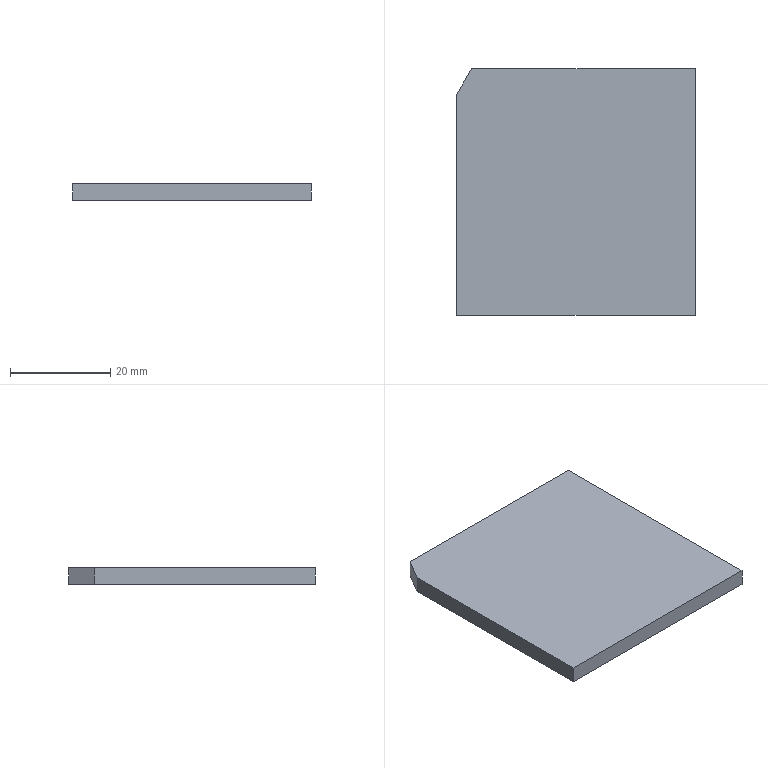Part | SolidWorks | features BaseBody 1 | 1 solid | 7 faces | box 47.6 x 49.1 x 3.35 mm | volume 7804 mm3 | plane 7
STEP:
#1=CARTESIAN_POINT('',(23.8,-24.55,0.));
#2=VERTEX_POINT('',#1);
#3=CARTESIAN_POINT('',(23.8,24.55,0.));
#4=VERTEX_POINT('',#3);
#5=CARTESIAN_POINT('',(23.8,0.,0.));
#6=DIRECTION('',(0.,1.,0.));
#7=VECTOR('',#6,1000.);
#8=LINE('',#5,#7);
#9=EDGE_CURVE('',#2,#4,#8,.T.);
#10=ORIENTED_EDGE('',*,*,#9,.F.);
#11=CARTESIAN_POINT('',(-23.8,-24.55,0.));
#12=VERTEX_POINT('',#11);
#13=CARTESIAN_POINT('',(0.,-24.55,0.));
#14=DIRECTION('',(1.,0.,0.));
#15=VECTOR('',#14,1000.);
#16=LINE('',#13,#15);
#17=EDGE_CURVE('',#12,#2,#16,.T.);
#18=ORIENTED_EDGE('',*,*,#17,.F.);
#19=CARTESIAN_POINT('',(-23.8,19.55,0.));
#20=VERTEX_POINT('',#19);
#21=CARTESIAN_POINT('',(-23.8,0.,0.));
#22=DIRECTION('',(0.,-1.,0.));
#23=VECTOR('',#22,1000.);
#24=LINE('',#21,#23);
#25=EDGE_CURVE('',#20,#12,#24,.T.);
#26=ORIENTED_EDGE('',*,*,#25,.F.);
#27=CARTESIAN_POINT('',(-20.8,24.55,0.));
#28=VERTEX_POINT('',#27);
#29=CARTESIAN_POINT('',(-20.8,24.55,0.));
#30=DIRECTION('',(-0.5145,-0.8575,0.));
#31=VECTOR('',#30,1000.);
#32=LINE('',#29,#31);
#33=EDGE_CURVE('',#28,#20,#32,.T.);
#34=ORIENTED_EDGE('',*,*,#33,.F.);
#35=CARTESIAN_POINT('',(0.,24.55,0.));
#36=DIRECTION('',(-1.,0.,0.));
#37=VECTOR('',#36,1000.);
#38=LINE('',#35,#37);
#39=EDGE_CURVE('',#4,#28,#38,.T.);
#40=ORIENTED_EDGE('',*,*,#39,.F.);
#41=EDGE_LOOP('',(#10,#18,#26,#34,#40));
#42=FACE_OUTER_BOUND('',#41,.T.);
#43=CARTESIAN_POINT('',(0.,0.,0.));
#44=DIRECTION('',(0.,0.,1.));
#45=DIRECTION('',(1.,0.,0.));
#46=AXIS2_PLACEMENT_3D('',#43,#44,#45);
#47=PLANE('',#46);
#48=ADVANCED_FACE('',(#42),#47,.F.);
#49=CARTESIAN_POINT('',(23.8,24.55,3.35));
#50=VERTEX_POINT('',#49);
#51=CARTESIAN_POINT('',(23.8,24.55,0.));
#52=DIRECTION('',(0.,0.,-1.));
#53=VECTOR('',#52,1000.);
#54=LINE('',#51,#53);
#55=EDGE_CURVE('',#50,#4,#54,.T.);
#56=ORIENTED_EDGE('',*,*,#55,.T.);
#57=ORIENTED_EDGE('',*,*,#39,.T.);
#58=CARTESIAN_POINT('',(-20.8,24.55,3.35));
#59=VERTEX_POINT('',#58);
#60=CARTESIAN_POINT('',(-20.8,24.55,0.));
#61=DIRECTION('',(0.,0.,1.));
#62=VECTOR('',#61,1000.);
#63=LINE('',#60,#62);
#64=EDGE_CURVE('',#28,#59,#63,.T.);
#65=ORIENTED_EDGE('',*,*,#64,.T.);
#66=CARTESIAN_POINT('',(23.8,24.55,3.35));
#67=DIRECTION('',(1.,0.,0.));
#68=VECTOR('',#67,1000.);
#69=LINE('',#66,#68);
#70=EDGE_CURVE('',#59,#50,#69,.T.);
#71=ORIENTED_EDGE('',*,*,#70,.T.);
#72=EDGE_LOOP('',(#56,#57,#65,#71));
#73=FACE_OUTER_BOUND('',#72,.T.);
#74=CARTESIAN_POINT('',(23.8,24.55,0.));
#75=DIRECTION('',(0.,1.,0.));
#76=DIRECTION('',(0.,0.,1.));
#77=AXIS2_PLACEMENT_3D('',#74,#75,#76);
#78=PLANE('',#77);
#79=ADVANCED_FACE('',(#73),#78,.T.);
#80=CARTESIAN_POINT('',(23.8,-24.55,3.35));
#81=VERTEX_POINT('',#80);
#82=CARTESIAN_POINT('',(23.8,-24.55,0.));
#83=DIRECTION('',(0.,0.,-1.));
#84=VECTOR('',#83,1000.);
#85=LINE('',#82,#84);
#86=EDGE_CURVE('',#81,#2,#85,.T.);
#87=ORIENTED_EDGE('',*,*,#86,.T.);
#88=ORIENTED_EDGE('',*,*,#9,.T.);
#89=ORIENTED_EDGE('',*,*,#55,.F.);
#90=CARTESIAN_POINT('',(23.8,-24.55,3.35));
#91=DIRECTION('',(0.,-1.,0.));
#92=VECTOR('',#91,1000.);
#93=LINE('',#90,#92);
#94=EDGE_CURVE('',#50,#81,#93,.T.);
#95=ORIENTED_EDGE('',*,*,#94,.T.);
#96=EDGE_LOOP('',(#87,#88,#89,#95));
#97=FACE_OUTER_BOUND('',#96,.T.);
#98=CARTESIAN_POINT('',(23.8,-24.55,0.));
#99=DIRECTION('',(1.,0.,0.));
#100=DIRECTION('',(0.,0.,-1.));
#101=AXIS2_PLACEMENT_3D('',#98,#99,#100);
#102=PLANE('',#101);
#103=ADVANCED_FACE('',(#97),#102,.T.);
#104=CARTESIAN_POINT('',(-23.8,-24.55,3.35));
#105=VERTEX_POINT('',#104);
#106=CARTESIAN_POINT('',(-23.8,-24.55,0.));
#107=DIRECTION('',(0.,0.,-1.));
#108=VECTOR('',#107,1000.);
#109=LINE('',#106,#108);
#110=EDGE_CURVE('',#105,#12,#109,.T.);
#111=ORIENTED_EDGE('',*,*,#110,.T.);
#112=ORIENTED_EDGE('',*,*,#17,.T.);
#113=ORIENTED_EDGE('',*,*,#86,.F.);
#114=CARTESIAN_POINT('',(-23.8,-24.55,3.35));
#115=DIRECTION('',(-1.,0.,0.));
#116=VECTOR('',#115,1000.);
#117=LINE('',#114,#116);
#118=EDGE_CURVE('',#81,#105,#117,.T.);
#119=ORIENTED_EDGE('',*,*,#118,.T.);
#120=EDGE_LOOP('',(#111,#112,#113,#119));
#121=FACE_OUTER_BOUND('',#120,.T.);
#122=CARTESIAN_POINT('',(-23.8,-24.55,0.));
#123=DIRECTION('',(0.,-1.,0.));
#124=DIRECTION('',(0.,0.,-1.));
#125=AXIS2_PLACEMENT_3D('',#122,#123,#124);
#126=PLANE('',#125);
#127=ADVANCED_FACE('',(#121),#126,.T.);
#128=CARTESIAN_POINT('',(-23.8,19.55,3.35));
#129=VERTEX_POINT('',#128);
#130=CARTESIAN_POINT('',(-23.8,19.55,0.));
#131=DIRECTION('',(0.,0.,-1.));
#132=VECTOR('',#131,1000.);
#133=LINE('',#130,#132);
#134=EDGE_CURVE('',#129,#20,#133,.T.);
#135=ORIENTED_EDGE('',*,*,#134,.T.);
#136=ORIENTED_EDGE('',*,*,#25,.T.);
#137=ORIENTED_EDGE('',*,*,#110,.F.);
#138=CARTESIAN_POINT('',(-23.8,19.55,3.35));
#139=DIRECTION('',(0.,1.,0.));
#140=VECTOR('',#139,1000.);
#141=LINE('',#138,#140);
#142=EDGE_CURVE('',#105,#129,#141,.T.);
#143=ORIENTED_EDGE('',*,*,#142,.T.);
#144=EDGE_LOOP('',(#135,#136,#137,#143));
#145=FACE_OUTER_BOUND('',#144,.T.);
#146=CARTESIAN_POINT('',(-23.8,19.55,0.));
#147=DIRECTION('',(-1.,0.,0.));
#148=DIRECTION('',(0.,0.,1.));
#149=AXIS2_PLACEMENT_3D('',#146,#147,#148);
#150=PLANE('',#149);
#151=ADVANCED_FACE('',(#145),#150,.T.);
#152=ORIENTED_EDGE('',*,*,#64,.F.);
#153=ORIENTED_EDGE('',*,*,#33,.T.);
#154=ORIENTED_EDGE('',*,*,#134,.F.);
#155=CARTESIAN_POINT('',(-20.8,24.55,3.35));
#156=DIRECTION('',(0.5145,0.8575,0.));
#157=VECTOR('',#156,1000.);
#158=LINE('',#155,#157);
#159=EDGE_CURVE('',#129,#59,#158,.T.);
#160=ORIENTED_EDGE('',*,*,#159,.T.);
#161=EDGE_LOOP('',(#152,#153,#154,#160));
#162=FACE_OUTER_BOUND('',#161,.T.);
#163=CARTESIAN_POINT('',(-20.8,24.55,0.));
#164=DIRECTION('',(-0.8575,0.5145,0.));
#165=DIRECTION('',(-0.5145,-0.8575,0.));
#166=AXIS2_PLACEMENT_3D('',#163,#164,#165);
#167=PLANE('',#166);
#168=ADVANCED_FACE('',(#162),#167,.T.);
#169=ORIENTED_EDGE('',*,*,#70,.F.);
#170=ORIENTED_EDGE('',*,*,#159,.F.);
#171=ORIENTED_EDGE('',*,*,#142,.F.);
#172=ORIENTED_EDGE('',*,*,#118,.F.);
#173=ORIENTED_EDGE('',*,*,#94,.F.);
#174=EDGE_LOOP('',(#169,#170,#171,#172,#173));
#175=FACE_OUTER_BOUND('',#174,.T.);
#176=CARTESIAN_POINT('',(0.,0.,3.35));
#177=DIRECTION('',(0.,0.,1.));
#178=DIRECTION('',(1.,0.,0.));
#179=AXIS2_PLACEMENT_3D('',#176,#177,#178);
#180=PLANE('',#179);
#181=ADVANCED_FACE('',(#175),#180,.T.);
#182=CLOSED_SHELL('',(#48,#79,#103,#127,#151,#168,#181));
#183=MANIFOLD_SOLID_BREP('',#182);
#184=CARTESIAN_POINT('',(0.,0.,0.));
#185=DIRECTION('',(0.,0.,1.));
#186=DIRECTION('',(1.,0.,0.));
#187=AXIS2_PLACEMENT_3D('',#184,#185,#186);
#188=(LENGTH_UNIT()NAMED_UNIT(*)SI_UNIT(.MILLI.,.METRE.));
#189=UNCERTAINTY_MEASURE_WITH_UNIT(LENGTH_MEASURE(0.00001),#188,'','');
#190=(NAMED_UNIT(*)PLANE_ANGLE_UNIT()SI_UNIT($,.RADIAN.));
#191=(NAMED_UNIT(*)SI_UNIT($,.STERADIAN.)SOLID_ANGLE_UNIT());
#192=(GEOMETRIC_REPRESENTATION_CONTEXT(3)GLOBAL_UNCERTAINTY_ASSIGNED_CONTEXT((#189))GLOBAL_UNIT_ASSIGNED_CONTEXT((#188,#190,#191))REPRESENTATION_CONTEXT('',''));
#193=ADVANCED_BREP_SHAPE_REPRESENTATION('',(#183,#187),#192);